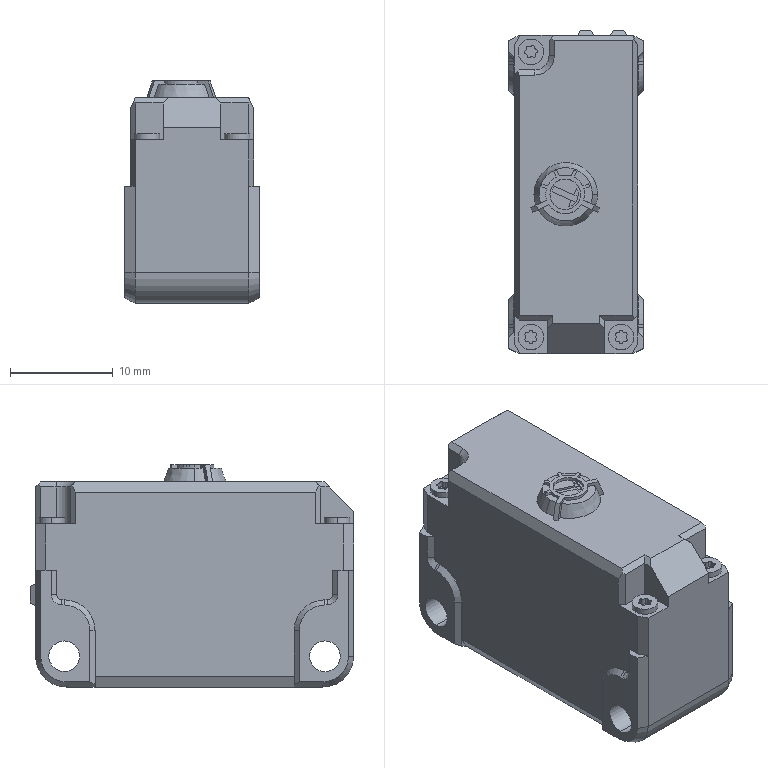Part | STEP file | PZ-G51EP-Part-2-13 | 1 solid | 229 faces | box 13.1 x 31.5 x 21.65 mm | volume 7160 mm3 | plane 128 | cylinder 84 | cone 17 | commonest cylinder face diameters 0.3 x25 0.5 x22 3.78 x7 2.5 x6 6 x6 1 x4